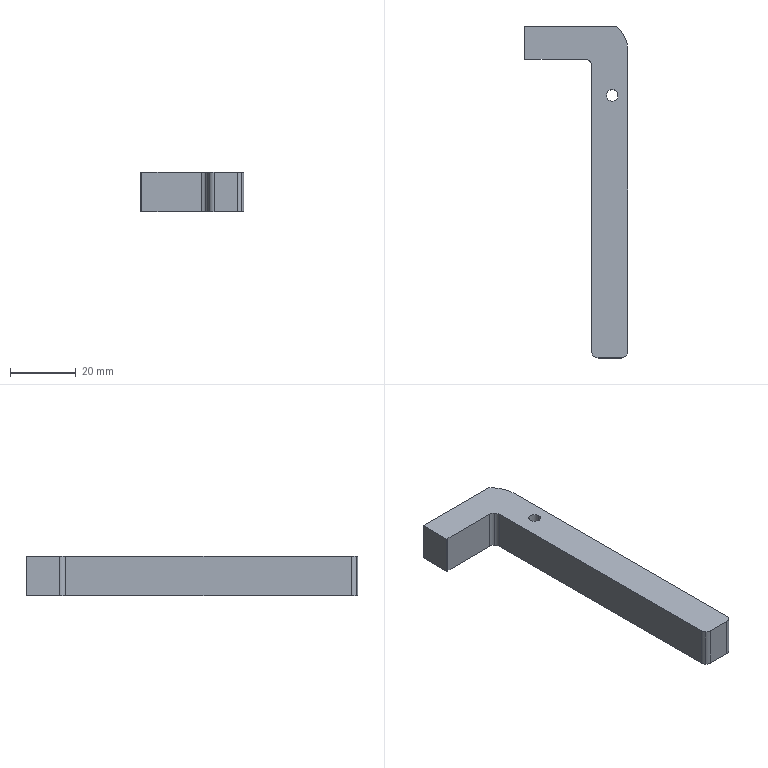Part | STEP file | ASND-0110-PWP TOP tu pang 20130814.sldasm-Part-7aq | 1 solid | 21 faces | box 31.546 x 101 x 12 mm | volume 15497 mm3 | cylinder 12 | plane 9 | commonest cylinder face diameters 4 x7 3.5 x2 6 x2 20 x1